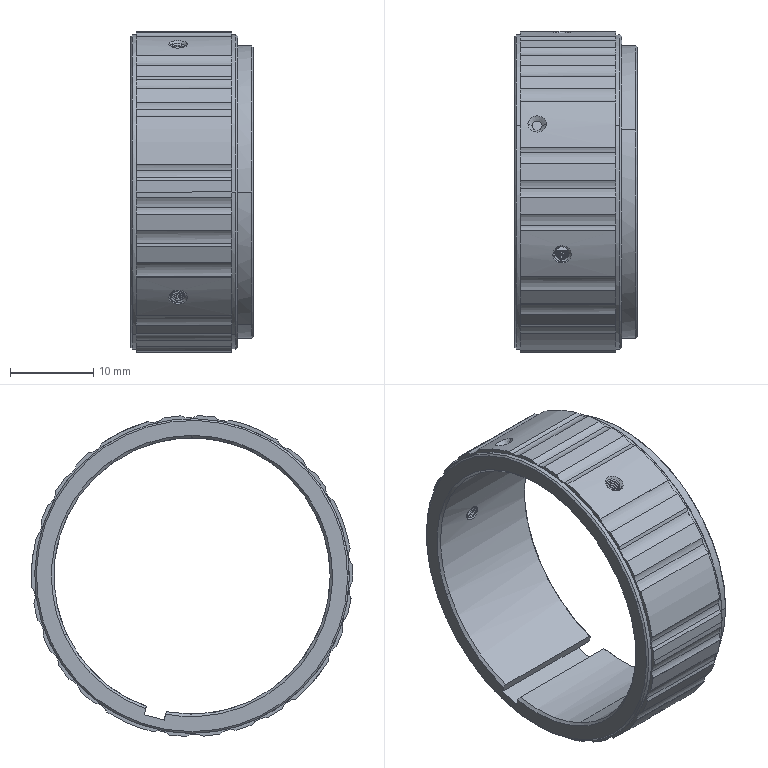Part | SolidWorks | features BaseBody 1 | 1 solid | 192 faces | box 14.76 x 38.6 x 38.577 mm | volume 3869 mm3 | cylinder 123 | spline 46 | cone 14 | plane 9 | commonest cylinder face diameters 1.6 x51 4 x36 38.6 x25 33.2 x4 35.2 x4 37.8 x3